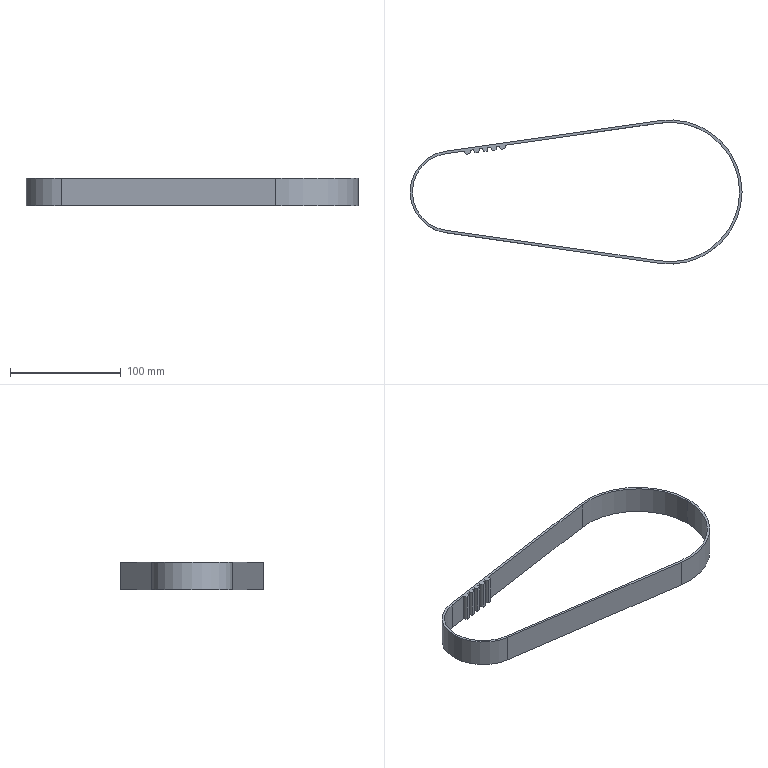Part | SolidWorks | features BaseBody 1 | 1 solid | 37 faces | box 300.461 x 130.452 x 25 mm | volume 41947 mm3 | cylinder 21 | plane 16 | commonest cylinder face diameters 10.4 x15 125.952 x2 130.452 x2 69.929 x1 74.429 x1
STEP:
#1=CARTESIAN_POINT('',(188.793,-64.57,-12.5));
#2=VERTEX_POINT('',#1);
#3=CARTESIAN_POINT('',(263.246,0.,-12.5));
#4=VERTEX_POINT('',#3);
#5=CARTESIAN_POINT('',(198.02,0.,-12.5));
#6=DIRECTION('',(0.,0.,1.));
#7=DIRECTION('',(1.,0.,0.));
#8=AXIS2_PLACEMENT_3D('',#5,#6,#7);
#9=CIRCLE('',#8,65.226);
#10=EDGE_CURVE('',#2,#4,#9,.T.);
#11=ORIENTED_EDGE('',*,*,#10,.T.);
#12=CARTESIAN_POINT('',(263.246,0.,12.5));
#13=VERTEX_POINT('',#12);
#14=CARTESIAN_POINT('',(263.246,0.,12.5));
#15=DIRECTION('',(0.,0.,1.));
#16=VECTOR('',#15,1000.);
#17=LINE('',#14,#16);
#18=EDGE_CURVE('',#4,#13,#17,.T.);
#19=ORIENTED_EDGE('',*,*,#18,.T.);
#20=CARTESIAN_POINT('',(188.793,-64.57,12.5));
#21=VERTEX_POINT('',#20);
#22=CARTESIAN_POINT('',(198.02,0.,12.5));
#23=DIRECTION('',(0.,0.,-1.));
#24=DIRECTION('',(1.,0.,0.));
#25=AXIS2_PLACEMENT_3D('',#22,#23,#24);
#26=CIRCLE('',#25,65.226);
#27=EDGE_CURVE('',#13,#21,#26,.T.);
#28=ORIENTED_EDGE('',*,*,#27,.T.);
#29=CARTESIAN_POINT('',(188.793,-64.57,12.5));
#30=DIRECTION('',(0.,0.,-1.));
#31=VECTOR('',#30,1000.);
#32=LINE('',#29,#31);
#33=EDGE_CURVE('',#21,#2,#32,.T.);
#34=ORIENTED_EDGE('',*,*,#33,.T.);
#35=EDGE_LOOP('',(#11,#19,#28,#34));
#36=FACE_OUTER_BOUND('',#35,.T.);
#37=CARTESIAN_POINT('',(198.02,0.,12.5));
#38=DIRECTION('',(0.,0.,1.));
#39=DIRECTION('',(1.,0.,0.));
#40=AXIS2_PLACEMENT_3D('',#37,#38,#39);
#41=CYLINDRICAL_SURFACE('',#40,65.226);
#42=ADVANCED_FACE('',(#36),#41,.T.);
#43=CARTESIAN_POINT('',(189.112,62.343,-12.5));
#44=VERTEX_POINT('',#43);
#45=CARTESIAN_POINT('',(260.996,0.,-12.5));
#46=VERTEX_POINT('',#45);
#47=CARTESIAN_POINT('',(198.02,0.,-12.5));
#48=DIRECTION('',(0.,0.,-1.));
#49=DIRECTION('',(1.,0.,0.));
#50=AXIS2_PLACEMENT_3D('',#47,#48,#49);
#51=CIRCLE('',#50,62.976);
#52=EDGE_CURVE('',#44,#46,#51,.T.);
#53=ORIENTED_EDGE('',*,*,#52,.T.);
#54=CARTESIAN_POINT('',(260.996,0.,12.5));
#55=VERTEX_POINT('',#54);
#56=CARTESIAN_POINT('',(260.996,0.,12.5));
#57=DIRECTION('',(0.,0.,1.));
#58=VECTOR('',#57,1000.);
#59=LINE('',#56,#58);
#60=EDGE_CURVE('',#46,#55,#59,.T.);
#61=ORIENTED_EDGE('',*,*,#60,.T.);
#62=CARTESIAN_POINT('',(189.112,62.343,12.5));
#63=VERTEX_POINT('',#62);
#64=CARTESIAN_POINT('',(198.02,0.,12.5));
#65=DIRECTION('',(0.,0.,-1.));
#66=DIRECTION('',(1.,0.,0.));
#67=AXIS2_PLACEMENT_3D('',#64,#65,#66);
#68=CIRCLE('',#67,62.976);
#69=EDGE_CURVE('',#63,#55,#68,.T.);
#70=ORIENTED_EDGE('',*,*,#69,.F.);
#71=CARTESIAN_POINT('',(189.112,62.343,12.5));
#72=DIRECTION('',(0.,0.,1.));
#73=VECTOR('',#72,1000.);
#74=LINE('',#71,#73);
#75=EDGE_CURVE('',#44,#63,#74,.T.);
#76=ORIENTED_EDGE('',*,*,#75,.F.);
#77=EDGE_LOOP('',(#53,#61,#70,#76));
#78=FACE_OUTER_BOUND('',#77,.T.);
#79=CARTESIAN_POINT('',(198.02,0.,12.5));
#80=DIRECTION('',(0.,0.,1.));
#81=DIRECTION('',(1.,0.,0.));
#82=AXIS2_PLACEMENT_3D('',#79,#80,#81);
#83=CYLINDRICAL_SURFACE('',#82,62.976);
#84=ADVANCED_FACE('',(#78),#83,.F.);
#85=CARTESIAN_POINT('',(48.558,39.178,-12.5));
#86=VERTEX_POINT('',#85);
#87=CARTESIAN_POINT('',(49.157,41.601,-12.5));
#88=VERTEX_POINT('',#87);
#89=CARTESIAN_POINT('',(43.957,41.601,-12.5));
#90=DIRECTION('',(0.,0.,1.));
#91=DIRECTION('',(1.,0.,0.));
#92=AXIS2_PLACEMENT_3D('',#89,#90,#91);
#93=CIRCLE('',#92,5.2);
#94=EDGE_CURVE('',#86,#88,#93,.T.);
#95=ORIENTED_EDGE('',*,*,#94,.T.);
#96=CARTESIAN_POINT('',(49.157,41.601,12.5));
#97=VERTEX_POINT('',#96);
#98=CARTESIAN_POINT('',(49.157,41.601,12.5));
#99=DIRECTION('',(0.,0.,1.));
#100=VECTOR('',#99,1000.);
#101=LINE('',#98,#100);
#102=EDGE_CURVE('',#88,#97,#101,.T.);
#103=ORIENTED_EDGE('',*,*,#102,.T.);
#104=CARTESIAN_POINT('',(48.558,39.178,12.5));
#105=VERTEX_POINT('',#104);
#106=CARTESIAN_POINT('',(43.957,41.601,12.5));
#107=DIRECTION('',(0.,0.,1.));
#108=DIRECTION('',(1.,0.,0.));
#109=AXIS2_PLACEMENT_3D('',#106,#107,#108);
#110=CIRCLE('',#109,5.2);
#111=EDGE_CURVE('',#105,#97,#110,.T.);
#112=ORIENTED_EDGE('',*,*,#111,.F.);
#113=CARTESIAN_POINT('',(48.558,39.178,12.5));
#114=DIRECTION('',(0.,0.,-1.));
#115=VECTOR('',#114,1000.);
#116=LINE('',#113,#115);
#117=EDGE_CURVE('',#105,#86,#116,.T.);
#118=ORIENTED_EDGE('',*,*,#117,.T.);
#119=EDGE_LOOP('',(#95,#103,#112,#118));
#120=FACE_OUTER_BOUND('',#119,.T.);
#121=CARTESIAN_POINT('',(43.957,41.601,12.5));
#122=DIRECTION('',(0.,0.,1.));
#123=DIRECTION('',(1.,0.,0.));
#124=AXIS2_PLACEMENT_3D('',#121,#122,#123);
#125=CYLINDRICAL_SURFACE('',#124,5.2);
#126=ADVANCED_FACE('',(#120),#125,.T.);
#127=CARTESIAN_POINT('',(40.638,38.046,-12.5));
#128=VERTEX_POINT('',#127);
#129=CARTESIAN_POINT('',(41.238,40.469,-12.5));
#130=VERTEX_POINT('',#129);
#131=CARTESIAN_POINT('',(36.038,40.469,-12.5));
#132=DIRECTION('',(0.,0.,1.));
#133=DIRECTION('',(1.,0.,0.));
#134=AXIS2_PLACEMENT_3D('',#131,#132,#133);
#135=CIRCLE('',#134,5.2);
#136=EDGE_CURVE('',#128,#130,#135,.T.);
#137=ORIENTED_EDGE('',*,*,#136,.T.);
#138=CARTESIAN_POINT('',(41.238,40.469,12.5));
#139=VERTEX_POINT('',#138);
#140=CARTESIAN_POINT('',(41.238,40.469,12.5));
#141=DIRECTION('',(0.,0.,1.));
#142=VECTOR('',#141,1000.);
#143=LINE('',#140,#142);
#144=EDGE_CURVE('',#130,#139,#143,.T.);
#145=ORIENTED_EDGE('',*,*,#144,.T.);
#146=CARTESIAN_POINT('',(40.638,38.046,12.5));
#147=VERTEX_POINT('',#146);
#148=CARTESIAN_POINT('',(36.038,40.469,12.5));
#149=DIRECTION('',(0.,0.,1.));
#150=DIRECTION('',(1.,0.,0.));
#151=AXIS2_PLACEMENT_3D('',#148,#149,#150);
#152=CIRCLE('',#151,5.2);
#153=EDGE_CURVE('',#147,#139,#152,.T.);
#154=ORIENTED_EDGE('',*,*,#153,.F.);
#155=CARTESIAN_POINT('',(40.638,38.046,12.5));
#156=DIRECTION('',(0.,0.,-1.));
#157=VECTOR('',#156,1000.);
#158=LINE('',#155,#157);
#159=EDGE_CURVE('',#147,#128,#158,.T.);
#160=ORIENTED_EDGE('',*,*,#159,.T.);
#161=EDGE_LOOP('',(#137,#145,#154,#160));
#162=FACE_OUTER_BOUND('',#161,.T.);
#163=CARTESIAN_POINT('',(36.038,40.469,12.5));
#164=DIRECTION('',(0.,0.,1.));
#165=DIRECTION('',(1.,0.,0.));
#166=AXIS2_PLACEMENT_3D('',#163,#164,#165);
#167=CYLINDRICAL_SURFACE('',#166,5.2);
#168=ADVANCED_FACE('',(#162),#167,.T.);
#169=CARTESIAN_POINT('',(32.719,36.914,-12.5));
#170=VERTEX_POINT('',#169);
#171=CARTESIAN_POINT('',(33.318,39.338,-12.5));
#172=VERTEX_POINT('',#171);
#173=CARTESIAN_POINT('',(28.118,39.338,-12.5));
#174=DIRECTION('',(0.,0.,1.));
#175=DIRECTION('',(1.,0.,0.));
#176=AXIS2_PLACEMENT_3D('',#173,#174,#175);
#177=CIRCLE('',#176,5.2);
#178=EDGE_CURVE('',#170,#172,#177,.T.);
#179=ORIENTED_EDGE('',*,*,#178,.T.);
#180=CARTESIAN_POINT('',(33.318,39.338,12.5));
#181=VERTEX_POINT('',#180);
#182=CARTESIAN_POINT('',(33.318,39.338,12.5));
#183=DIRECTION('',(0.,0.,1.));
#184=VECTOR('',#183,1000.);
#185=LINE('',#182,#184);
#186=EDGE_CURVE('',#172,#181,#185,.T.);
#187=ORIENTED_EDGE('',*,*,#186,.T.);
#188=CARTESIAN_POINT('',(32.719,36.914,12.5));
#189=VERTEX_POINT('',#188);
#190=CARTESIAN_POINT('',(28.118,39.338,12.5));
#191=DIRECTION('',(0.,0.,1.));
#192=DIRECTION('',(1.,0.,0.));
#193=AXIS2_PLACEMENT_3D('',#190,#191,#192);
#194=CIRCLE('',#193,5.2);
#195=EDGE_CURVE('',#189,#181,#194,.T.);
#196=ORIENTED_EDGE('',*,*,#195,.F.);
#197=CARTESIAN_POINT('',(32.719,36.914,12.5));
#198=DIRECTION('',(0.,0.,-1.));
#199=VECTOR('',#198,1000.);
#200=LINE('',#197,#199);
#201=EDGE_CURVE('',#189,#170,#200,.T.);
#202=ORIENTED_EDGE('',*,*,#201,.T.);
#203=EDGE_LOOP('',(#179,#187,#196,#202));
#204=FACE_OUTER_BOUND('',#203,.T.);
#205=CARTESIAN_POINT('',(28.118,39.338,12.5));
#206=DIRECTION('',(0.,0.,1.));
#207=DIRECTION('',(1.,0.,0.));
#208=AXIS2_PLACEMENT_3D('',#205,#206,#207);
#209=CYLINDRICAL_SURFACE('',#208,5.2);
#210=ADVANCED_FACE('',(#204),#209,.T.);
#211=CARTESIAN_POINT('',(24.799,35.783,-12.5));
#212=VERTEX_POINT('',#211);
#213=CARTESIAN_POINT('',(25.399,38.206,-12.5));
#214=VERTEX_POINT('',#213);
#215=CARTESIAN_POINT('',(20.199,38.206,-12.5));
#216=DIRECTION('',(0.,0.,1.));
#217=DIRECTION('',(1.,0.,0.));
#218=AXIS2_PLACEMENT_3D('',#215,#216,#217);
#219=CIRCLE('',#218,5.2);
#220=EDGE_CURVE('',#212,#214,#219,.T.);
#221=ORIENTED_EDGE('',*,*,#220,.T.);
#222=CARTESIAN_POINT('',(25.399,38.206,12.5));
#223=VERTEX_POINT('',#222);
#224=CARTESIAN_POINT('',(25.399,38.206,12.5));
#225=DIRECTION('',(0.,0.,1.));
#226=VECTOR('',#225,1000.);
#227=LINE('',#224,#226);
#228=EDGE_CURVE('',#214,#223,#227,.T.);
#229=ORIENTED_EDGE('',*,*,#228,.T.);
#230=CARTESIAN_POINT('',(24.799,35.783,12.5));
#231=VERTEX_POINT('',#230);
#232=CARTESIAN_POINT('',(20.199,38.206,12.5));
#233=DIRECTION('',(0.,0.,1.));
#234=DIRECTION('',(1.,0.,0.));
#235=AXIS2_PLACEMENT_3D('',#232,#233,#234);
#236=CIRCLE('',#235,5.2);
#237=EDGE_CURVE('',#231,#223,#236,.T.);
#238=ORIENTED_EDGE('',*,*,#237,.F.);
#239=CARTESIAN_POINT('',(24.799,35.783,12.5));
#240=DIRECTION('',(0.,0.,-1.));
#241=VECTOR('',#240,1000.);
#242=LINE('',#239,#241);
#243=EDGE_CURVE('',#231,#212,#242,.T.);
#244=ORIENTED_EDGE('',*,*,#243,.T.);
#245=EDGE_LOOP('',(#221,#229,#238,#244));
#246=FACE_OUTER_BOUND('',#245,.T.);
#247=CARTESIAN_POINT('',(20.199,38.206,12.5));
#248=DIRECTION('',(0.,0.,1.));
#249=DIRECTION('',(1.,0.,0.));
#250=AXIS2_PLACEMENT_3D('',#247,#248,#249);
#251=CYLINDRICAL_SURFACE('',#250,5.2);
#252=ADVANCED_FACE('',(#246),#251,.T.);
#253=CARTESIAN_POINT('',(16.88,34.651,-12.5));
#254=VERTEX_POINT('',#253);
#255=CARTESIAN_POINT('',(17.479,37.074,-12.5));
#256=VERTEX_POINT('',#255);
#257=CARTESIAN_POINT('',(12.279,37.074,-12.5));
#258=DIRECTION('',(0.,0.,1.));
#259=DIRECTION('',(1.,0.,0.));
#260=AXIS2_PLACEMENT_3D('',#257,#258,#259);
#261=CIRCLE('',#260,5.2);
#262=EDGE_CURVE('',#254,#256,#261,.T.);
#263=ORIENTED_EDGE('',*,*,#262,.T.);
#264=CARTESIAN_POINT('',(17.479,37.074,12.5));
#265=VERTEX_POINT('',#264);
#266=CARTESIAN_POINT('',(17.479,37.074,12.5));
#267=DIRECTION('',(0.,0.,1.));
#268=VECTOR('',#267,1000.);
#269=LINE('',#266,#268);
#270=EDGE_CURVE('',#256,#265,#269,.T.);
#271=ORIENTED_EDGE('',*,*,#270,.T.);
#272=CARTESIAN_POINT('',(16.88,34.651,12.5));
#273=VERTEX_POINT('',#272);
#274=CARTESIAN_POINT('',(12.279,37.074,12.5));
#275=DIRECTION('',(0.,0.,1.));
#276=DIRECTION('',(1.,0.,0.));
#277=AXIS2_PLACEMENT_3D('',#274,#275,#276);
#278=CIRCLE('',#277,5.2);
#279=EDGE_CURVE('',#273,#265,#278,.T.);
#280=ORIENTED_EDGE('',*,*,#279,.F.);
#281=CARTESIAN_POINT('',(16.88,34.651,12.5));
#282=DIRECTION('',(0.,0.,-1.));
#283=VECTOR('',#282,1000.);
#284=LINE('',#281,#283);
#285=EDGE_CURVE('',#273,#254,#284,.T.);
#286=ORIENTED_EDGE('',*,*,#285,.T.);
#287=EDGE_LOOP('',(#263,#271,#280,#286));
#288=FACE_OUTER_BOUND('',#287,.T.);
#289=CARTESIAN_POINT('',(12.279,37.074,12.5));
#290=DIRECTION('',(0.,0.,1.));
#291=DIRECTION('',(1.,0.,0.));
#292=AXIS2_PLACEMENT_3D('',#289,#290,#291);
#293=CYLINDRICAL_SURFACE('',#292,5.2);
#294=ADVANCED_FACE('',(#288),#293,.T.);
#295=ORIENTED_EDGE('',*,*,#18,.F.);
#296=CARTESIAN_POINT('',(188.793,64.57,-12.5));
#297=VERTEX_POINT('',#296);
#298=CARTESIAN_POINT('',(198.02,0.,-12.5));
#299=DIRECTION('',(0.,0.,1.));
#300=DIRECTION('',(1.,0.,0.));
#301=AXIS2_PLACEMENT_3D('',#298,#299,#300);
#302=CIRCLE('',#301,65.226);
#303=EDGE_CURVE('',#4,#297,#302,.T.);
#304=ORIENTED_EDGE('',*,*,#303,.T.);
#305=CARTESIAN_POINT('',(188.793,64.57,12.5));
#306=VERTEX_POINT('',#305);
#307=CARTESIAN_POINT('',(188.793,64.57,12.5));
#308=DIRECTION('',(0.,0.,1.));
#309=VECTOR('',#308,1000.);
#310=LINE('',#307,#309);
#311=EDGE_CURVE('',#297,#306,#310,.T.);
#312=ORIENTED_EDGE('',*,*,#311,.T.);
#313=CARTESIAN_POINT('',(198.02,0.,12.5));
#314=DIRECTION('',(0.,0.,-1.));
#315=DIRECTION('',(1.,0.,0.));
#316=AXIS2_PLACEMENT_3D('',#313,#314,#315);
#317=CIRCLE('',#316,65.226);
#318=EDGE_CURVE('',#306,#13,#317,.T.);
#319=ORIENTED_EDGE('',*,*,#318,.T.);
#320=EDGE_LOOP('',(#295,#304,#312,#319));
#321=FACE_OUTER_BOUND('',#320,.T.);
#322=CARTESIAN_POINT('',(198.02,0.,12.5));
#323=DIRECTION('',(0.,0.,1.));
#324=DIRECTION('',(1.,0.,0.));
#325=AXIS2_PLACEMENT_3D('',#322,#323,#324);
#326=CYLINDRICAL_SURFACE('',#325,65.226);
#327=ADVANCED_FACE('',(#321),#326,.T.);
#328=ORIENTED_EDGE('',*,*,#33,.F.);
#329=CARTESIAN_POINT('',(-5.264,-36.84,12.5));
#330=VERTEX_POINT('',#329);
#331=CARTESIAN_POINT('',(-5.264,-36.84,12.5));
#332=DIRECTION('',(0.9899,-0.1415,0.));
#333=VECTOR('',#332,1000.);
#334=LINE('',#331,#333);
#335=EDGE_CURVE('',#330,#21,#334,.T.);
#336=ORIENTED_EDGE('',*,*,#335,.F.);
#337=CARTESIAN_POINT('',(-5.264,-36.84,-12.5));
#338=VERTEX_POINT('',#337);
#339=CARTESIAN_POINT('',(-5.264,-36.84,12.5));
#340=DIRECTION('',(0.,0.,1.));
#341=VECTOR('',#340,1000.);
#342=LINE('',#339,#341);
#343=EDGE_CURVE('',#338,#330,#342,.T.);
#344=ORIENTED_EDGE('',*,*,#343,.F.);
#345=CARTESIAN_POINT('',(-5.264,-36.84,-12.5));
#346=DIRECTION('',(-0.9899,0.1415,0.));
#347=VECTOR('',#346,1000.);
#348=LINE('',#345,#347);
#349=EDGE_CURVE('',#2,#338,#348,.T.);
#350=ORIENTED_EDGE('',*,*,#349,.F.);
#351=EDGE_LOOP('',(#328,#336,#344,#350));
#352=FACE_OUTER_BOUND('',#351,.T.);
#353=CARTESIAN_POINT('',(-5.264,-36.84,12.5));
#354=DIRECTION('',(0.1415,0.9899,0.));
#355=DIRECTION('',(-0.9899,0.1415,0.));
#356=AXIS2_PLACEMENT_3D('',#353,#354,#355);
#357=PLANE('',#356);
#358=ADVANCED_FACE('',(#352),#357,.F.);
#359=CARTESIAN_POINT('',(189.112,-62.343,12.5));
#360=VERTEX_POINT('',#359);
#361=CARTESIAN_POINT('',(-4.946,-34.613,12.5));
#362=VERTEX_POINT('',#361);
#363=CARTESIAN_POINT('',(189.112,-62.343,12.5));
#364=DIRECTION('',(-0.9899,0.1415,0.));
#365=VECTOR('',#364,1000.);
#366=LINE('',#363,#365);
#367=EDGE_CURVE('',#360,#362,#366,.T.);
#368=ORIENTED_EDGE('',*,*,#367,.T.);
#369=CARTESIAN_POINT('',(-4.946,34.613,12.5));
#370=VERTEX_POINT('',#369);
#371=CARTESIAN_POINT('',(0.,0.,12.5));
#372=DIRECTION('',(0.,0.,-1.));
#373=DIRECTION('',(1.,0.,0.));
#374=AXIS2_PLACEMENT_3D('',#371,#372,#373);
#375=CIRCLE('',#374,34.965);
#376=EDGE_CURVE('',#362,#370,#375,.T.);
#377=ORIENTED_EDGE('',*,*,#376,.T.);
#378=CARTESIAN_POINT('',(12.279,37.074,12.5));
#379=VERTEX_POINT('',#378);
#380=CARTESIAN_POINT('',(-4.946,34.613,12.5));
#381=DIRECTION('',(0.9899,0.1415,0.));
#382=VECTOR('',#381,1000.);
#383=LINE('',#380,#382);
#384=EDGE_CURVE('',#370,#379,#383,.T.);
#385=ORIENTED_EDGE('',*,*,#384,.T.);
#386=CARTESIAN_POINT('',(13.689,34.195,12.5));
#387=VERTEX_POINT('',#386);
#388=CARTESIAN_POINT('',(17.427,37.81,12.5));
#389=DIRECTION('',(0.,0.,1.));
#390=DIRECTION('',(1.,0.,0.));
#391=AXIS2_PLACEMENT_3D('',#388,#389,#390);
#392=CIRCLE('',#391,5.2);
#393=EDGE_CURVE('',#379,#387,#392,.T.);
#394=ORIENTED_EDGE('',*,*,#393,.T.);
#395=CARTESIAN_POINT('',(13.689,34.195,12.5));
#396=DIRECTION('',(0.9899,0.1415,0.));
#397=VECTOR('',#396,1000.);
#398=LINE('',#395,#397);
#399=EDGE_CURVE('',#387,#273,#398,.T.);
#400=ORIENTED_EDGE('',*,*,#399,.T.);
#401=ORIENTED_EDGE('',*,*,#279,.T.);
#402=CARTESIAN_POINT('',(17.427,37.81,12.5));
#403=VERTEX_POINT('',#402);
#404=CARTESIAN_POINT('',(12.279,37.074,12.5));
#405=DIRECTION('',(0.,0.,1.));
#406=DIRECTION('',(1.,0.,0.));
#407=AXIS2_PLACEMENT_3D('',#404,#405,#406);
#408=CIRCLE('',#407,5.2);
#409=EDGE_CURVE('',#265,#403,#408,.T.);
#410=ORIENTED_EDGE('',*,*,#409,.T.);
#411=CARTESIAN_POINT('',(20.199,38.206,12.5));
#412=VERTEX_POINT('',#411);
#413=CARTESIAN_POINT('',(17.427,37.81,12.5));
#414=DIRECTION('',(0.9899,0.1415,0.));
#415=VECTOR('',#414,1000.);
#416=LINE('',#413,#415);
#417=EDGE_CURVE('',#403,#412,#416,.T.);
#418=ORIENTED_EDGE('',*,*,#417,.T.);
#419=CARTESIAN_POINT('',(21.609,35.327,12.5));
#420=VERTEX_POINT('',#419);
#421=CARTESIAN_POINT('',(25.346,38.942,12.5));
#422=DIRECTION('',(0.,0.,1.));
#423=DIRECTION('',(1.,0.,0.));
#424=AXIS2_PLACEMENT_3D('',#421,#422,#423);
#425=CIRCLE('',#424,5.2);
#426=EDGE_CURVE('',#412,#420,#425,.T.);
#427=ORIENTED_EDGE('',*,*,#426,.T.);
#428=CARTESIAN_POINT('',(21.609,35.327,12.5));
#429=DIRECTION('',(0.9899,0.1415,0.));
#430=VECTOR('',#429,1000.);
#431=LINE('',#428,#430);
#432=EDGE_CURVE('',#420,#231,#431,.T.);
#433=ORIENTED_EDGE('',*,*,#432,.T.);
#434=ORIENTED_EDGE('',*,*,#237,.T.);
#435=CARTESIAN_POINT('',(25.346,38.942,12.5));
#436=VERTEX_POINT('',#435);
#437=CARTESIAN_POINT('',(20.199,38.206,12.5));
#438=DIRECTION('',(0.,0.,1.));
#439=DIRECTION('',(1.,0.,0.));
#440=AXIS2_PLACEMENT_3D('',#437,#438,#439);
#441=CIRCLE('',#440,5.2);
#442=EDGE_CURVE('',#223,#436,#441,.T.);
#443=ORIENTED_EDGE('',*,*,#442,.T.);
#444=CARTESIAN_POINT('',(28.118,39.338,12.5));
#445=VERTEX_POINT('',#444);
#446=CARTESIAN_POINT('',(25.346,38.942,12.5));
#447=DIRECTION('',(0.9899,0.1415,0.));
#448=VECTOR('',#447,1000.);
#449=LINE('',#446,#448);
#450=EDGE_CURVE('',#436,#445,#449,.T.);
#451=ORIENTED_EDGE('',*,*,#450,.T.);
#452=CARTESIAN_POINT('',(29.528,36.458,12.5));
#453=VERTEX_POINT('',#452);
#454=CARTESIAN_POINT('',(33.266,40.073,12.5));
#455=DIRECTION('',(0.,0.,1.));
#456=DIRECTION('',(1.,0.,0.));
#457=AXIS2_PLACEMENT_3D('',#454,#455,#456);
#458=CIRCLE('',#457,5.2);
#459=EDGE_CURVE('',#445,#453,#458,.T.);
#460=ORIENTED_EDGE('',*,*,#459,.T.);
#461=CARTESIAN_POINT('',(29.528,36.458,12.5));
#462=DIRECTION('',(0.9899,0.1415,0.));
#463=VECTOR('',#462,1000.);
#464=LINE('',#461,#463);
#465=EDGE_CURVE('',#453,#189,#464,.T.);
#466=ORIENTED_EDGE('',*,*,#465,.T.);
#467=ORIENTED_EDGE('',*,*,#195,.T.);
#468=CARTESIAN_POINT('',(33.266,40.073,12.5));
#469=VERTEX_POINT('',#468);
#470=CARTESIAN_POINT('',(28.118,39.338,12.5));
#471=DIRECTION('',(0.,0.,1.));
#472=DIRECTION('',(1.,0.,0.));
#473=AXIS2_PLACEMENT_3D('',#470,#471,#472);
#474=CIRCLE('',#473,5.2);
#475=EDGE_CURVE('',#181,#469,#474,.T.);
#476=ORIENTED_EDGE('',*,*,#475,.T.);
#477=CARTESIAN_POINT('',(36.038,40.469,12.5));
#478=VERTEX_POINT('',#477);
#479=CARTESIAN_POINT('',(33.266,40.073,12.5));
#480=DIRECTION('',(0.9899,0.1415,0.));
#481=VECTOR('',#480,1000.);
#482=LINE('',#479,#481);
#483=EDGE_CURVE('',#469,#478,#482,.T.);
#484=ORIENTED_EDGE('',*,*,#483,.T.);
#485=CARTESIAN_POINT('',(37.448,37.59,12.5));
#486=VERTEX_POINT('',#485);
#487=CARTESIAN_POINT('',(41.185,41.205,12.5));
#488=DIRECTION('',(0.,0.,1.));
#489=DIRECTION('',(1.,0.,0.));
#490=AXIS2_PLACEMENT_3D('',#487,#488,#489);
#491=CIRCLE('',#490,5.2);
#492=EDGE_CURVE('',#478,#486,#491,.T.);
#493=ORIENTED_EDGE('',*,*,#492,.T.);
#494=CARTESIAN_POINT('',(37.448,37.59,12.5));
#495=DIRECTION('',(0.9899,0.1415,0.));
#496=VECTOR('',#495,1000.);
#497=LINE('',#494,#496);
#498=EDGE_CURVE('',#486,#147,#497,.T.);
#499=ORIENTED_EDGE('',*,*,#498,.T.);
#500=ORIENTED_EDGE('',*,*,#153,.T.);
#501=CARTESIAN_POINT('',(41.185,41.205,12.5));
#502=VERTEX_POINT('',#501);
#503=CARTESIAN_POINT('',(36.038,40.469,12.5));
#504=DIRECTION('',(0.,0.,1.));
#505=DIRECTION('',(1.,0.,0.));
#506=AXIS2_PLACEMENT_3D('',#503,#504,#505);
#507=CIRCLE('',#506,5.2);
#508=EDGE_CURVE('',#139,#502,#507,.T.);
#509=ORIENTED_EDGE('',*,*,#508,.T.);
#510=CARTESIAN_POINT('',(43.957,41.601,12.5));
#511=VERTEX_POINT('',#510);
#512=CARTESIAN_POINT('',(41.185,41.205,12.5));
#513=DIRECTION('',(0.9899,0.1415,0.));
#514=VECTOR('',#513,1000.);
#515=LINE('',#512,#514);
#516=EDGE_CURVE('',#502,#511,#515,.T.);
#517=ORIENTED_EDGE('',*,*,#516,.T.);
#518=CARTESIAN_POINT('',(45.367,38.722,12.5));
#519=VERTEX_POINT('',#518);
#520=CARTESIAN_POINT('',(49.105,42.337,12.5));
#521=DIRECTION('',(0.,0.,1.));
#522=DIRECTION('',(1.,0.,0.));
#523=AXIS2_PLACEMENT_3D('',#520,#521,#522);
#524=CIRCLE('',#523,5.2);
#525=EDGE_CURVE('',#511,#519,#524,.T.);
#526=ORIENTED_EDGE('',*,*,#525,.T.);
#527=CARTESIAN_POINT('',(45.367,38.722,12.5));
#528=DIRECTION('',(0.9899,0.1415,0.));
#529=VECTOR('',#528,1000.);
#530=LINE('',#527,#529);
#531=EDGE_CURVE('',#519,#105,#530,.T.);
#532=ORIENTED_EDGE('',*,*,#531,.T.);
#533=ORIENTED_EDGE('',*,*,#111,.T.);
#534=CARTESIAN_POINT('',(49.105,42.337,12.5));
#535=VERTEX_POINT('',#534);
#536=CARTESIAN_POINT('',(43.957,41.601,12.5));
#537=DIRECTION('',(0.,0.,1.));
#538=DIRECTION('',(1.,0.,0.));
#539=AXIS2_PLACEMENT_3D('',#536,#537,#538);
#540=CIRCLE('',#539,5.2);
#541=EDGE_CURVE('',#97,#535,#540,.T.);
#542=ORIENTED_EDGE('',*,*,#541,.T.);
#543=CARTESIAN_POINT('',(49.105,42.337,12.5));
#544=DIRECTION('',(0.9899,0.1415,0.));
#545=VECTOR('',#544,1000.);
#546=LINE('',#543,#545);
#547=EDGE_CURVE('',#535,#63,#546,.T.);
#548=ORIENTED_EDGE('',*,*,#547,.T.);
#549=ORIENTED_EDGE('',*,*,#69,.T.);
#550=CARTESIAN_POINT('',(198.02,0.,12.5));
#551=DIRECTION('',(0.,0.,-1.));
#552=DIRECTION('',(1.,0.,0.));
#553=AXIS2_PLACEMENT_3D('',#550,#551,#552);
#554=CIRCLE('',#553,62.976);
#555=EDGE_CURVE('',#55,#360,#554,.T.);
#556=ORIENTED_EDGE('',*,*,#555,.T.);
#557=EDGE_LOOP('',(#368,#377,#385,#394,#400,#401,#410,#418,#427,#433,#434,#443,#451,#460,#466,#467,#476,#484,#493,#499,#500,#509,#517,#526,#532,#533,#542,#548,#549,#556));
#558=FACE_BOUND('',#557,.T.);
#559=ORIENTED_EDGE('',*,*,#335,.T.);
#560=ORIENTED_EDGE('',*,*,#27,.F.);
#561=ORIENTED_EDGE('',*,*,#318,.F.);
#562=CARTESIAN_POINT('',(-5.264,36.84,12.5));
#563=VERTEX_POINT('',#562);
#564=CARTESIAN_POINT('',(188.793,64.57,12.5));
#565=DIRECTION('',(-0.9899,-0.1415,0.));
#566=VECTOR('',#565,1000.);
#567=LINE('',#564,#566);
#568=EDGE_CURVE('',#306,#563,#567,.T.);
#569=ORIENTED_EDGE('',*,*,#568,.T.);
#570=CARTESIAN_POINT('',(0.,0.,12.5));
#571=DIRECTION('',(0.,0.,1.));
#572=DIRECTION('',(1.,0.,0.));
#573=AXIS2_PLACEMENT_3D('',#570,#571,#572);
#574=CIRCLE('',#573,37.215);
#575=EDGE_CURVE('',#563,#330,#574,.T.);
#576=ORIENTED_EDGE('',*,*,#575,.T.);
#577=EDGE_LOOP('',(#559,#560,#561,#569,#576));
#578=FACE_OUTER_BOUND('',#577,.T.);
#579=CARTESIAN_POINT('',(17.427,37.81,12.5));
#580=DIRECTION('',(0.,0.,1.));
#581=DIRECTION('',(1.,0.,0.));
#582=AXIS2_PLACEMENT_3D('',#579,#580,#581);
#583=PLANE('',#582);
#584=ADVANCED_FACE('',(#558,#578),#583,.T.);
#585=CARTESIAN_POINT('',(-5.264,36.84,-12.5));
#586=VERTEX_POINT('',#585);
#587=CARTESIAN_POINT('',(-5.264,36.84,12.5));
#588=DIRECTION('',(0.,0.,-1.));
#589=VECTOR('',#588,1000.);
#590=LINE('',#587,#589);
#591=EDGE_CURVE('',#563,#586,#590,.T.);
#592=ORIENTED_EDGE('',*,*,#591,.F.);
#593=ORIENTED_EDGE('',*,*,#568,.F.);
#594=ORIENTED_EDGE('',*,*,#311,.F.);
#595=CARTESIAN_POINT('',(50.173,44.762,-12.5));
#596=DIRECTION('',(0.9899,0.1415,0.));
#597=VECTOR('',#596,1000.);
#598=LINE('',#595,#597);
#599=EDGE_CURVE('',#586,#297,#598,.T.);
#600=ORIENTED_EDGE('',*,*,#599,.F.);
#601=EDGE_LOOP('',(#592,#593,#594,#600));
#602=FACE_OUTER_BOUND('',#601,.T.);
#603=CARTESIAN_POINT('',(50.173,44.762,12.5));
#604=DIRECTION('',(0.1415,-0.9899,0.));
#605=DIRECTION('',(0.9899,0.1415,0.));
#606=AXIS2_PLACEMENT_3D('',#603,#604,#605);
#607=PLANE('',#606);
#608=ADVANCED_FACE('',(#602),#607,.F.);
#609=CARTESIAN_POINT('',(-4.946,-34.613,-12.5));
#610=VERTEX_POINT('',#609);
#611=CARTESIAN_POINT('',(-4.946,34.613,-12.5));
#612=VERTEX_POINT('',#611);
#613=CARTESIAN_POINT('',(0.,0.,-12.5));
#614=DIRECTION('',(0.,0.,-1.));
#615=DIRECTION('',(1.,0.,0.));
#616=AXIS2_PLACEMENT_3D('',#613,#614,#615);
#617=CIRCLE('',#616,34.965);
#618=EDGE_CURVE('',#610,#612,#617,.T.);
#619=ORIENTED_EDGE('',*,*,#618,.F.);
#620=CARTESIAN_POINT('',(189.112,-62.343,-12.5));
#621=VERTEX_POINT('',#620);
#622=CARTESIAN_POINT('',(189.112,-62.343,-12.5));
#623=DIRECTION('',(-0.9899,0.1415,0.));
#624=VECTOR('',#623,1000.);
#625=LINE('',#622,#624);
#626=EDGE_CURVE('',#621,#610,#625,.T.);
#627=ORIENTED_EDGE('',*,*,#626,.F.);
#628=CARTESIAN_POINT('',(198.02,0.,-12.5));
#629=DIRECTION('',(0.,0.,-1.));
#630=DIRECTION('',(1.,0.,0.));
#631=AXIS2_PLACEMENT_3D('',#628,#629,#630);
#632=CIRCLE('',#631,62.976);
#633=EDGE_CURVE('',#46,#621,#632,.T.);
#634=ORIENTED_EDGE('',*,*,#633,.F.);
#635=ORIENTED_EDGE('',*,*,#52,.F.);
#636=CARTESIAN_POINT('',(49.105,42.337,-12.5));
#637=VERTEX_POINT('',#636);
#638=CARTESIAN_POINT('',(49.105,42.337,-12.5));
#639=DIRECTION('',(0.9899,0.1415,0.));
#640=VECTOR('',#639,1000.);
#641=LINE('',#638,#640);
#642=EDGE_CURVE('',#637,#44,#641,.T.);
#643=ORIENTED_EDGE('',*,*,#642,.F.);
#644=CARTESIAN_POINT('',(43.957,41.601,-12.5));
#645=DIRECTION('',(0.,0.,1.));
#646=DIRECTION('',(1.,0.,0.));
#647=AXIS2_PLACEMENT_3D('',#644,#645,#646);
#648=CIRCLE('',#647,5.2);
#649=EDGE_CURVE('',#88,#637,#648,.T.);
#650=ORIENTED_EDGE('',*,*,#649,.F.);
#651=ORIENTED_EDGE('',*,*,#94,.F.);
#652=CARTESIAN_POINT('',(45.367,38.722,-12.5));
#653=VERTEX_POINT('',#652);
#654=CARTESIAN_POINT('',(45.367,38.722,-12.5));
#655=DIRECTION('',(0.9899,0.1415,0.));
#656=VECTOR('',#655,1000.);
#657=LINE('',#654,#656);
#658=EDGE_CURVE('',#653,#86,#657,.T.);
#659=ORIENTED_EDGE('',*,*,#658,.F.);
#660=CARTESIAN_POINT('',(43.957,41.601,-12.5));
#661=VERTEX_POINT('',#660);
#662=CARTESIAN_POINT('',(49.105,42.337,-12.5));
#663=DIRECTION('',(0.,0.,1.));
#664=DIRECTION('',(1.,0.,0.));
#665=AXIS2_PLACEMENT_3D('',#662,#663,#664);
#666=CIRCLE('',#665,5.2);
#667=EDGE_CURVE('',#661,#653,#666,.T.);
#668=ORIENTED_EDGE('',*,*,#667,.F.);
#669=CARTESIAN_POINT('',(41.185,41.205,-12.5));
#670=VERTEX_POINT('',#669);
#671=CARTESIAN_POINT('',(41.185,41.205,-12.5));
#672=DIRECTION('',(0.9899,0.1415,0.));
#673=VECTOR('',#672,1000.);
#674=LINE('',#671,#673);
#675=EDGE_CURVE('',#670,#661,#674,.T.);
#676=ORIENTED_EDGE('',*,*,#675,.F.);
#677=CARTESIAN_POINT('',(36.038,40.469,-12.5));
#678=DIRECTION('',(0.,0.,1.));
#679=DIRECTION('',(1.,0.,0.));
#680=AXIS2_PLACEMENT_3D('',#677,#678,#679);
#681=CIRCLE('',#680,5.2);
#682=EDGE_CURVE('',#130,#670,#681,.T.);
#683=ORIENTED_EDGE('',*,*,#682,.F.);
#684=ORIENTED_EDGE('',*,*,#136,.F.);
#685=CARTESIAN_POINT('',(37.448,37.59,-12.5));
#686=VERTEX_POINT('',#685);
#687=CARTESIAN_POINT('',(37.448,37.59,-12.5));
#688=DIRECTION('',(0.9899,0.1415,0.));
#689=VECTOR('',#688,1000.);
#690=LINE('',#687,#689);
#691=EDGE_CURVE('',#686,#128,#690,.T.);
#692=ORIENTED_EDGE('',*,*,#691,.F.);
#693=CARTESIAN_POINT('',(36.038,40.469,-12.5));
#694=VERTEX_POINT('',#693);
#695=CARTESIAN_POINT('',(41.185,41.205,-12.5));
#696=DIRECTION('',(0.,0.,1.));
#697=DIRECTION('',(1.,0.,0.));
#698=AXIS2_PLACEMENT_3D('',#695,#696,#697);
#699=CIRCLE('',#698,5.2);
#700=EDGE_CURVE('',#694,#686,#699,.T.);
#701=ORIENTED_EDGE('',*,*,#700,.F.);
#702=CARTESIAN_POINT('',(33.266,40.073,-12.5));
#703=VERTEX_POINT('',#702);
#704=CARTESIAN_POINT('',(33.266,40.073,-12.5));
#705=DIRECTION('',(0.9899,0.1415,0.));
#706=VECTOR('',#705,1000.);
#707=LINE('',#704,#706);
#708=EDGE_CURVE('',#703,#694,#707,.T.);
#709=ORIENTED_EDGE('',*,*,#708,.F.);
#710=CARTESIAN_POINT('',(28.118,39.338,-12.5));
#711=DIRECTION('',(0.,0.,1.));
#712=DIRECTION('',(1.,0.,0.));
#713=AXIS2_PLACEMENT_3D('',#710,#711,#712);
#714=CIRCLE('',#713,5.2);
#715=EDGE_CURVE('',#172,#703,#714,.T.);
#716=ORIENTED_EDGE('',*,*,#715,.F.);
#717=ORIENTED_EDGE('',*,*,#178,.F.);
#718=CARTESIAN_POINT('',(29.528,36.458,-12.5));
#719=VERTEX_POINT('',#718);
#720=CARTESIAN_POINT('',(29.528,36.458,-12.5));
#721=DIRECTION('',(0.9899,0.1415,0.));
#722=VECTOR('',#721,1000.);
#723=LINE('',#720,#722);
#724=EDGE_CURVE('',#719,#170,#723,.T.);
#725=ORIENTED_EDGE('',*,*,#724,.F.);
#726=CARTESIAN_POINT('',(28.118,39.338,-12.5));
#727=VERTEX_POINT('',#726);
#728=CARTESIAN_POINT('',(33.266,40.073,-12.5));
#729=DIRECTION('',(0.,0.,1.));
#730=DIRECTION('',(1.,0.,0.));
#731=AXIS2_PLACEMENT_3D('',#728,#729,#730);
#732=CIRCLE('',#731,5.2);
#733=EDGE_CURVE('',#727,#719,#732,.T.);
#734=ORIENTED_EDGE('',*,*,#733,.F.);
#735=CARTESIAN_POINT('',(25.346,38.942,-12.5));
#736=VERTEX_POINT('',#735);
#737=CARTESIAN_POINT('',(25.346,38.942,-12.5));
#738=DIRECTION('',(0.9899,0.1415,0.));
#739=VECTOR('',#738,1000.);
#740=LINE('',#737,#739);
#741=EDGE_CURVE('',#736,#727,#740,.T.);
#742=ORIENTED_EDGE('',*,*,#741,.F.);
#743=CARTESIAN_POINT('',(20.199,38.206,-12.5));
#744=DIRECTION('',(0.,0.,1.));
#745=DIRECTION('',(1.,0.,0.));
#746=AXIS2_PLACEMENT_3D('',#743,#744,#745);
#747=CIRCLE('',#746,5.2);
#748=EDGE_CURVE('',#214,#736,#747,.T.);
#749=ORIENTED_EDGE('',*,*,#748,.F.);
#750=ORIENTED_EDGE('',*,*,#220,.F.);
#751=CARTESIAN_POINT('',(21.609,35.327,-12.5));
#752=VERTEX_POINT('',#751);
#753=CARTESIAN_POINT('',(21.609,35.327,-12.5));
#754=DIRECTION('',(0.9899,0.1415,0.));
#755=VECTOR('',#754,1000.);
#756=LINE('',#753,#755);
#757=EDGE_CURVE('',#752,#212,#756,.T.);
#758=ORIENTED_EDGE('',*,*,#757,.F.);
#759=CARTESIAN_POINT('',(20.199,38.206,-12.5));
#760=VERTEX_POINT('',#759);
#761=CARTESIAN_POINT('',(25.346,38.942,-12.5));
#762=DIRECTION('',(0.,0.,1.));
#763=DIRECTION('',(1.,0.,0.));
#764=AXIS2_PLACEMENT_3D('',#761,#762,#763);
#765=CIRCLE('',#764,5.2);
#766=EDGE_CURVE('',#760,#752,#765,.T.);
#767=ORIENTED_EDGE('',*,*,#766,.F.);
#768=CARTESIAN_POINT('',(17.427,37.81,-12.5));
#769=VERTEX_POINT('',#768);
#770=CARTESIAN_POINT('',(17.427,37.81,-12.5));
#771=DIRECTION('',(0.9899,0.1415,0.));
#772=VECTOR('',#771,1000.);
#773=LINE('',#770,#772);
#774=EDGE_CURVE('',#769,#760,#773,.T.);
#775=ORIENTED_EDGE('',*,*,#774,.F.);
#776=CARTESIAN_POINT('',(12.279,37.074,-12.5));
#777=DIRECTION('',(0.,0.,1.));
#778=DIRECTION('',(1.,0.,0.));
#779=AXIS2_PLACEMENT_3D('',#776,#777,#778);
#780=CIRCLE('',#779,5.2);
#781=EDGE_CURVE('',#256,#769,#780,.T.);
#782=ORIENTED_EDGE('',*,*,#781,.F.);
#783=ORIENTED_EDGE('',*,*,#262,.F.);
#784=CARTESIAN_POINT('',(13.689,34.195,-12.5));
#785=VERTEX_POINT('',#784);
#786=CARTESIAN_POINT('',(13.689,34.195,-12.5));
#787=DIRECTION('',(0.9899,0.1415,0.));
#788=VECTOR('',#787,1000.);
#789=LINE('',#786,#788);
#790=EDGE_CURVE('',#785,#254,#789,.T.);
#791=ORIENTED_EDGE('',*,*,#790,.F.);
#792=CARTESIAN_POINT('',(12.279,37.074,-12.5));
#793=VERTEX_POINT('',#792);
#794=CARTESIAN_POINT('',(17.427,37.81,-12.5));
#795=DIRECTION('',(0.,0.,1.));
#796=DIRECTION('',(1.,0.,0.));
#797=AXIS2_PLACEMENT_3D('',#794,#795,#796);
#798=CIRCLE('',#797,5.2);
#799=EDGE_CURVE('',#793,#785,#798,.T.);
#800=ORIENTED_EDGE('',*,*,#799,.F.);
#801=CARTESIAN_POINT('',(-4.946,34.613,-12.5));
#802=DIRECTION('',(0.9899,0.1415,0.));
#803=VECTOR('',#802,1000.);
#804=LINE('',#801,#803);
#805=EDGE_CURVE('',#612,#793,#804,.T.);
#806=ORIENTED_EDGE('',*,*,#805,.F.);
#807=EDGE_LOOP('',(#619,#627,#634,#635,#643,#650,#651,#659,#668,#676,#683,#684,#692,#701,#709,#716,#717,#725,#734,#742,#749,#750,#758,#767,#775,#782,#783,#791,#800,#806));
#808=FACE_BOUND('',#807,.T.);
#809=ORIENTED_EDGE('',*,*,#599,.T.);
#810=ORIENTED_EDGE('',*,*,#303,.F.);
#811=ORIENTED_EDGE('',*,*,#10,.F.);
#812=ORIENTED_EDGE('',*,*,#349,.T.);
#813=CARTESIAN_POINT('',(0.,0.,-12.5));
#814=DIRECTION('',(0.,0.,1.));
#815=DIRECTION('',(1.,0.,0.));
#816=AXIS2_PLACEMENT_3D('',#813,#814,#815);
#817=CIRCLE('',#816,37.215);
#818=EDGE_CURVE('',#586,#338,#817,.T.);
#819=ORIENTED_EDGE('',*,*,#818,.F.);
#820=EDGE_LOOP('',(#809,#810,#811,#812,#819));
#821=FACE_OUTER_BOUND('',#820,.T.);
#822=CARTESIAN_POINT('',(17.427,37.81,-12.5));
#823=DIRECTION('',(0.,0.,1.));
#824=DIRECTION('',(1.,0.,0.));
#825=AXIS2_PLACEMENT_3D('',#822,#823,#824);
#826=PLANE('',#825);
#827=ADVANCED_FACE('',(#808,#821),#826,.F.);
#828=ORIENTED_EDGE('',*,*,#343,.T.);
#829=ORIENTED_EDGE('',*,*,#575,.F.);
#830=ORIENTED_EDGE('',*,*,#591,.T.);
#831=ORIENTED_EDGE('',*,*,#818,.T.);
#832=EDGE_LOOP('',(#828,#829,#830,#831));
#833=FACE_OUTER_BOUND('',#832,.T.);
#834=CARTESIAN_POINT('',(0.,0.,12.5));
#835=DIRECTION('',(0.,0.,1.));
#836=DIRECTION('',(1.,0.,0.));
#837=AXIS2_PLACEMENT_3D('',#834,#835,#836);
#838=CYLINDRICAL_SURFACE('',#837,37.215);
#839=ADVANCED_FACE('',(#833),#838,.T.);
#840=CARTESIAN_POINT('',(-4.946,-34.613,12.5));
#841=DIRECTION('',(0.,0.,1.));
#842=VECTOR('',#841,1000.);
#843=LINE('',#840,#842);
#844=EDGE_CURVE('',#610,#362,#843,.T.);
#845=ORIENTED_EDGE('',*,*,#844,.F.);
#846=ORIENTED_EDGE('',*,*,#618,.T.);
#847=CARTESIAN_POINT('',(-4.946,34.613,12.5));
#848=DIRECTION('',(0.,0.,1.));
#849=VECTOR('',#848,1000.);
#850=LINE('',#847,#849);
#851=EDGE_CURVE('',#612,#370,#850,.T.);
#852=ORIENTED_EDGE('',*,*,#851,.T.);
#853=ORIENTED_EDGE('',*,*,#376,.F.);
#854=EDGE_LOOP('',(#845,#846,#852,#853));
#855=FACE_OUTER_BOUND('',#854,.T.);
#856=CARTESIAN_POINT('',(0.,0.,12.5));
#857=DIRECTION('',(0.,0.,1.));
#858=DIRECTION('',(1.,0.,0.));
#859=AXIS2_PLACEMENT_3D('',#856,#857,#858);
#860=CYLINDRICAL_SURFACE('',#859,34.965);
#861=ADVANCED_FACE('',(#855),#860,.F.);
#862=ORIENTED_EDGE('',*,*,#367,.F.);
#863=CARTESIAN_POINT('',(189.112,-62.343,12.5));
#864=DIRECTION('',(0.,0.,-1.));
#865=VECTOR('',#864,1000.);
#866=LINE('',#863,#865);
#867=EDGE_CURVE('',#360,#621,#866,.T.);
#868=ORIENTED_EDGE('',*,*,#867,.T.);
#869=ORIENTED_EDGE('',*,*,#626,.T.);
#870=ORIENTED_EDGE('',*,*,#844,.T.);
#871=EDGE_LOOP('',(#862,#868,#869,#870));
#872=FACE_OUTER_BOUND('',#871,.T.);
#873=CARTESIAN_POINT('',(-4.946,-34.613,12.5));
#874=DIRECTION('',(0.1415,0.9899,0.));
#875=DIRECTION('',(-0.9899,0.1415,0.));
#876=AXIS2_PLACEMENT_3D('',#873,#874,#875);
#877=PLANE('',#876);
#878=ADVANCED_FACE('',(#872),#877,.T.);
#879=ORIENTED_EDGE('',*,*,#60,.F.);
#880=ORIENTED_EDGE('',*,*,#633,.T.);
#881=ORIENTED_EDGE('',*,*,#867,.F.);
#882=ORIENTED_EDGE('',*,*,#555,.F.);
#883=EDGE_LOOP('',(#879,#880,#881,#882));
#884=FACE_OUTER_BOUND('',#883,.T.);
#885=CARTESIAN_POINT('',(198.02,0.,12.5));
#886=DIRECTION('',(0.,0.,1.));
#887=DIRECTION('',(1.,0.,0.));
#888=AXIS2_PLACEMENT_3D('',#885,#886,#887);
#889=CYLINDRICAL_SURFACE('',#888,62.976);
#890=ADVANCED_FACE('',(#884),#889,.F.);
#891=ORIENTED_EDGE('',*,*,#75,.T.);
#892=ORIENTED_EDGE('',*,*,#547,.F.);
#893=CARTESIAN_POINT('',(49.105,42.337,12.5));
#894=DIRECTION('',(0.,0.,1.));
#895=VECTOR('',#894,1000.);
#896=LINE('',#893,#895);
#897=EDGE_CURVE('',#637,#535,#896,.T.);
#898=ORIENTED_EDGE('',*,*,#897,.F.);
#899=ORIENTED_EDGE('',*,*,#642,.T.);
#900=EDGE_LOOP('',(#891,#892,#898,#899));
#901=FACE_OUTER_BOUND('',#900,.T.);
#902=CARTESIAN_POINT('',(49.105,42.337,12.5));
#903=DIRECTION('',(-0.1415,0.9899,0.));
#904=DIRECTION('',(-0.9899,-0.1415,0.));
#905=AXIS2_PLACEMENT_3D('',#902,#903,#904);
#906=PLANE('',#905);
#907=ADVANCED_FACE('',(#901),#906,.F.);
#908=ORIENTED_EDGE('',*,*,#102,.F.);
#909=ORIENTED_EDGE('',*,*,#649,.T.);
#910=ORIENTED_EDGE('',*,*,#897,.T.);
#911=ORIENTED_EDGE('',*,*,#541,.F.);
#912=EDGE_LOOP('',(#908,#909,#910,#911));
#913=FACE_OUTER_BOUND('',#912,.T.);
#914=CARTESIAN_POINT('',(43.957,41.601,12.5));
#915=DIRECTION('',(0.,0.,1.));
#916=DIRECTION('',(1.,0.,0.));
#917=AXIS2_PLACEMENT_3D('',#914,#915,#916);
#918=CYLINDRICAL_SURFACE('',#917,5.2);
#919=ADVANCED_FACE('',(#913),#918,.T.);
#920=ORIENTED_EDGE('',*,*,#117,.F.);
#921=ORIENTED_EDGE('',*,*,#531,.F.);
#922=CARTESIAN_POINT('',(45.367,38.722,12.5));
#923=DIRECTION('',(0.,0.,1.));
#924=VECTOR('',#923,1000.);
#925=LINE('',#922,#924);
#926=EDGE_CURVE('',#653,#519,#925,.T.);
#927=ORIENTED_EDGE('',*,*,#926,.F.);
#928=ORIENTED_EDGE('',*,*,#658,.T.);
#929=EDGE_LOOP('',(#920,#921,#927,#928));
#930=FACE_OUTER_BOUND('',#929,.T.);
#931=CARTESIAN_POINT('',(45.367,38.722,12.5));
#932=DIRECTION('',(-0.1415,0.9899,0.));
#933=DIRECTION('',(-0.9899,-0.1415,0.));
#934=AXIS2_PLACEMENT_3D('',#931,#932,#933);
#935=PLANE('',#934);
#936=ADVANCED_FACE('',(#930),#935,.F.);
#937=ORIENTED_EDGE('',*,*,#525,.F.);
#938=CARTESIAN_POINT('',(43.957,41.601,12.5));
#939=DIRECTION('',(0.,0.,-1.));
#940=VECTOR('',#939,1000.);
#941=LINE('',#938,#940);
#942=EDGE_CURVE('',#511,#661,#941,.T.);
#943=ORIENTED_EDGE('',*,*,#942,.T.);
#944=ORIENTED_EDGE('',*,*,#667,.T.);
#945=ORIENTED_EDGE('',*,*,#926,.T.);
#946=EDGE_LOOP('',(#937,#943,#944,#945));
#947=FACE_OUTER_BOUND('',#946,.T.);
#948=CARTESIAN_POINT('',(49.105,42.337,12.5));
#949=DIRECTION('',(0.,0.,1.));
#950=DIRECTION('',(1.,0.,0.));
#951=AXIS2_PLACEMENT_3D('',#948,#949,#950);
#952=CYLINDRICAL_SURFACE('',#951,5.2);
#953=ADVANCED_FACE('',(#947),#952,.T.);
#954=ORIENTED_EDGE('',*,*,#942,.F.);
#955=ORIENTED_EDGE('',*,*,#516,.F.);
#956=CARTESIAN_POINT('',(41.185,41.205,12.5));
#957=DIRECTION('',(0.,0.,1.));
#958=VECTOR('',#957,1000.);
#959=LINE('',#956,#958);
#960=EDGE_CURVE('',#670,#502,#959,.T.);
#961=ORIENTED_EDGE('',*,*,#960,.F.);
#962=ORIENTED_EDGE('',*,*,#675,.T.);
#963=EDGE_LOOP('',(#954,#955,#961,#962));
#964=FACE_OUTER_BOUND('',#963,.T.);
#965=CARTESIAN_POINT('',(41.185,41.205,12.5));
#966=DIRECTION('',(-0.1415,0.9899,0.));
#967=DIRECTION('',(-0.9899,-0.1415,0.));
#968=AXIS2_PLACEMENT_3D('',#965,#966,#967);
#969=PLANE('',#968);
#970=ADVANCED_FACE('',(#964),#969,.F.);
#971=ORIENTED_EDGE('',*,*,#144,.F.);
#972=ORIENTED_EDGE('',*,*,#682,.T.);
#973=ORIENTED_EDGE('',*,*,#960,.T.);
#974=ORIENTED_EDGE('',*,*,#508,.F.);
#975=EDGE_LOOP('',(#971,#972,#973,#974));
#976=FACE_OUTER_BOUND('',#975,.T.);
#977=CARTESIAN_POINT('',(36.038,40.469,12.5));
#978=DIRECTION('',(0.,0.,1.));
#979=DIRECTION('',(1.,0.,0.));
#980=AXIS2_PLACEMENT_3D('',#977,#978,#979);
#981=CYLINDRICAL_SURFACE('',#980,5.2);
#982=ADVANCED_FACE('',(#976),#981,.T.);
#983=ORIENTED_EDGE('',*,*,#159,.F.);
#984=ORIENTED_EDGE('',*,*,#498,.F.);
#985=CARTESIAN_POINT('',(37.448,37.59,12.5));
#986=DIRECTION('',(0.,0.,1.));
#987=VECTOR('',#986,1000.);
#988=LINE('',#985,#987);
#989=EDGE_CURVE('',#686,#486,#988,.T.);
#990=ORIENTED_EDGE('',*,*,#989,.F.);
#991=ORIENTED_EDGE('',*,*,#691,.T.);
#992=EDGE_LOOP('',(#983,#984,#990,#991));
#993=FACE_OUTER_BOUND('',#992,.T.);
#994=CARTESIAN_POINT('',(37.448,37.59,12.5));
#995=DIRECTION('',(-0.1415,0.9899,0.));
#996=DIRECTION('',(-0.9899,-0.1415,0.));
#997=AXIS2_PLACEMENT_3D('',#994,#995,#996);
#998=PLANE('',#997);
#999=ADVANCED_FACE('',(#993),#998,.F.);
#1000=ORIENTED_EDGE('',*,*,#492,.F.);
#1001=CARTESIAN_POINT('',(36.038,40.469,12.5));
#1002=DIRECTION('',(0.,0.,-1.));
#1003=VECTOR('',#1002,1000.);
#1004=LINE('',#1001,#1003);
#1005=EDGE_CURVE('',#478,#694,#1004,.T.);
#1006=ORIENTED_EDGE('',*,*,#1005,.T.);
#1007=ORIENTED_EDGE('',*,*,#700,.T.);
#1008=ORIENTED_EDGE('',*,*,#989,.T.);
#1009=EDGE_LOOP('',(#1000,#1006,#1007,#1008));
#1010=FACE_OUTER_BOUND('',#1009,.T.);
#1011=CARTESIAN_POINT('',(41.185,41.205,12.5));
#1012=DIRECTION('',(0.,0.,1.));
#1013=DIRECTION('',(1.,0.,0.));
#1014=AXIS2_PLACEMENT_3D('',#1011,#1012,#1013);
#1015=CYLINDRICAL_SURFACE('',#1014,5.2);
#1016=ADVANCED_FACE('',(#1010),#1015,.T.);
#1017=ORIENTED_EDGE('',*,*,#1005,.F.);
#1018=ORIENTED_EDGE('',*,*,#483,.F.);
#1019=CARTESIAN_POINT('',(33.266,40.073,12.5));
#1020=DIRECTION('',(0.,0.,1.));
#1021=VECTOR('',#1020,1000.);
#1022=LINE('',#1019,#1021);
#1023=EDGE_CURVE('',#703,#469,#1022,.T.);
#1024=ORIENTED_EDGE('',*,*,#1023,.F.);
#1025=ORIENTED_EDGE('',*,*,#708,.T.);
#1026=EDGE_LOOP('',(#1017,#1018,#1024,#1025));
#1027=FACE_OUTER_BOUND('',#1026,.T.);
#1028=CARTESIAN_POINT('',(33.266,40.073,12.5));
#1029=DIRECTION('',(-0.1415,0.9899,0.));
#1030=DIRECTION('',(-0.9899,-0.1415,0.));
#1031=AXIS2_PLACEMENT_3D('',#1028,#1029,#1030);
#1032=PLANE('',#1031);
#1033=ADVANCED_FACE('',(#1027),#1032,.F.);
#1034=ORIENTED_EDGE('',*,*,#186,.F.);
#1035=ORIENTED_EDGE('',*,*,#715,.T.);
#1036=ORIENTED_EDGE('',*,*,#1023,.T.);
#1037=ORIENTED_EDGE('',*,*,#475,.F.);
#1038=EDGE_LOOP('',(#1034,#1035,#1036,#1037));
#1039=FACE_OUTER_BOUND('',#1038,.T.);
#1040=CARTESIAN_POINT('',(28.118,39.338,12.5));
#1041=DIRECTION('',(0.,0.,1.));
#1042=DIRECTION('',(1.,0.,0.));
#1043=AXIS2_PLACEMENT_3D('',#1040,#1041,#1042);
#1044=CYLINDRICAL_SURFACE('',#1043,5.2);
#1045=ADVANCED_FACE('',(#1039),#1044,.T.);
#1046=ORIENTED_EDGE('',*,*,#201,.F.);
#1047=ORIENTED_EDGE('',*,*,#465,.F.);
#1048=CARTESIAN_POINT('',(29.528,36.458,12.5));
#1049=DIRECTION('',(0.,0.,1.));
#1050=VECTOR('',#1049,1000.);
#1051=LINE('',#1048,#1050);
#1052=EDGE_CURVE('',#719,#453,#1051,.T.);
#1053=ORIENTED_EDGE('',*,*,#1052,.F.);
#1054=ORIENTED_EDGE('',*,*,#724,.T.);
#1055=EDGE_LOOP('',(#1046,#1047,#1053,#1054));
#1056=FACE_OUTER_BOUND('',#1055,.T.);
#1057=CARTESIAN_POINT('',(29.528,36.458,12.5));
#1058=DIRECTION('',(-0.1415,0.9899,0.));
#1059=DIRECTION('',(-0.9899,-0.1415,0.));
#1060=AXIS2_PLACEMENT_3D('',#1057,#1058,#1059);
#1061=PLANE('',#1060);
#1062=ADVANCED_FACE('',(#1056),#1061,.F.);
#1063=ORIENTED_EDGE('',*,*,#459,.F.);
#1064=CARTESIAN_POINT('',(28.118,39.338,12.5));
#1065=DIRECTION('',(0.,0.,-1.));
#1066=VECTOR('',#1065,1000.);
#1067=LINE('',#1064,#1066);
#1068=EDGE_CURVE('',#445,#727,#1067,.T.);
#1069=ORIENTED_EDGE('',*,*,#1068,.T.);
#1070=ORIENTED_EDGE('',*,*,#733,.T.);
#1071=ORIENTED_EDGE('',*,*,#1052,.T.);
#1072=EDGE_LOOP('',(#1063,#1069,#1070,#1071));
#1073=FACE_OUTER_BOUND('',#1072,.T.);
#1074=CARTESIAN_POINT('',(33.266,40.073,12.5));
#1075=DIRECTION('',(0.,0.,1.));
#1076=DIRECTION('',(1.,0.,0.));
#1077=AXIS2_PLACEMENT_3D('',#1074,#1075,#1076);
#1078=CYLINDRICAL_SURFACE('',#1077,5.2);
#1079=ADVANCED_FACE('',(#1073),#1078,.T.);
#1080=ORIENTED_EDGE('',*,*,#1068,.F.);
#1081=ORIENTED_EDGE('',*,*,#450,.F.);
#1082=CARTESIAN_POINT('',(25.346,38.942,12.5));
#1083=DIRECTION('',(0.,0.,1.));
#1084=VECTOR('',#1083,1000.);
#1085=LINE('',#1082,#1084);
#1086=EDGE_CURVE('',#736,#436,#1085,.T.);
#1087=ORIENTED_EDGE('',*,*,#1086,.F.);
#1088=ORIENTED_EDGE('',*,*,#741,.T.);
#1089=EDGE_LOOP('',(#1080,#1081,#1087,#1088));
#1090=FACE_OUTER_BOUND('',#1089,.T.);
#1091=CARTESIAN_POINT('',(25.346,38.942,12.5));
#1092=DIRECTION('',(-0.1415,0.9899,0.));
#1093=DIRECTION('',(-0.9899,-0.1415,0.));
#1094=AXIS2_PLACEMENT_3D('',#1091,#1092,#1093);
#1095=PLANE('',#1094);
#1096=ADVANCED_FACE('',(#1090),#1095,.F.);
#1097=ORIENTED_EDGE('',*,*,#228,.F.);
#1098=ORIENTED_EDGE('',*,*,#748,.T.);
#1099=ORIENTED_EDGE('',*,*,#1086,.T.);
#1100=ORIENTED_EDGE('',*,*,#442,.F.);
#1101=EDGE_LOOP('',(#1097,#1098,#1099,#1100));
#1102=FACE_OUTER_BOUND('',#1101,.T.);
#1103=CARTESIAN_POINT('',(20.199,38.206,12.5));
#1104=DIRECTION('',(0.,0.,1.));
#1105=DIRECTION('',(1.,0.,0.));
#1106=AXIS2_PLACEMENT_3D('',#1103,#1104,#1105);
#1107=CYLINDRICAL_SURFACE('',#1106,5.2);
#1108=ADVANCED_FACE('',(#1102),#1107,.T.);
#1109=ORIENTED_EDGE('',*,*,#243,.F.);
#1110=ORIENTED_EDGE('',*,*,#432,.F.);
#1111=CARTESIAN_POINT('',(21.609,35.327,12.5));
#1112=DIRECTION('',(0.,0.,1.));
#1113=VECTOR('',#1112,1000.);
#1114=LINE('',#1111,#1113);
#1115=EDGE_CURVE('',#752,#420,#1114,.T.);
#1116=ORIENTED_EDGE('',*,*,#1115,.F.);
#1117=ORIENTED_EDGE('',*,*,#757,.T.);
#1118=EDGE_LOOP('',(#1109,#1110,#1116,#1117));
#1119=FACE_OUTER_BOUND('',#1118,.T.);
#1120=CARTESIAN_POINT('',(21.609,35.327,12.5));
#1121=DIRECTION('',(-0.1415,0.9899,0.));
#1122=DIRECTION('',(-0.9899,-0.1415,0.));
#1123=AXIS2_PLACEMENT_3D('',#1120,#1121,#1122);
#1124=PLANE('',#1123);
#1125=ADVANCED_FACE('',(#1119),#1124,.F.);
#1126=ORIENTED_EDGE('',*,*,#426,.F.);
#1127=CARTESIAN_POINT('',(20.199,38.206,12.5));
#1128=DIRECTION('',(0.,0.,-1.));
#1129=VECTOR('',#1128,1000.);
#1130=LINE('',#1127,#1129);
#1131=EDGE_CURVE('',#412,#760,#1130,.T.);
#1132=ORIENTED_EDGE('',*,*,#1131,.T.);
#1133=ORIENTED_EDGE('',*,*,#766,.T.);
#1134=ORIENTED_EDGE('',*,*,#1115,.T.);
#1135=EDGE_LOOP('',(#1126,#1132,#1133,#1134));
#1136=FACE_OUTER_BOUND('',#1135,.T.);
#1137=CARTESIAN_POINT('',(25.346,38.942,12.5));
#1138=DIRECTION('',(0.,0.,1.));
#1139=DIRECTION('',(1.,0.,0.));
#1140=AXIS2_PLACEMENT_3D('',#1137,#1138,#1139);
#1141=CYLINDRICAL_SURFACE('',#1140,5.2);
#1142=ADVANCED_FACE('',(#1136),#1141,.T.);
#1143=ORIENTED_EDGE('',*,*,#1131,.F.);
#1144=ORIENTED_EDGE('',*,*,#417,.F.);
#1145=CARTESIAN_POINT('',(17.427,37.81,12.5));
#1146=DIRECTION('',(0.,0.,1.));
#1147=VECTOR('',#1146,1000.);
#1148=LINE('',#1145,#1147);
#1149=EDGE_CURVE('',#769,#403,#1148,.T.);
#1150=ORIENTED_EDGE('',*,*,#1149,.F.);
#1151=ORIENTED_EDGE('',*,*,#774,.T.);
#1152=EDGE_LOOP('',(#1143,#1144,#1150,#1151));
#1153=FACE_OUTER_BOUND('',#1152,.T.);
#1154=CARTESIAN_POINT('',(17.427,37.81,12.5));
#1155=DIRECTION('',(-0.1415,0.9899,0.));
#1156=DIRECTION('',(-0.9899,-0.1415,0.));
#1157=AXIS2_PLACEMENT_3D('',#1154,#1155,#1156);
#1158=PLANE('',#1157);
#1159=ADVANCED_FACE('',(#1153),#1158,.F.);
#1160=ORIENTED_EDGE('',*,*,#270,.F.);
#1161=ORIENTED_EDGE('',*,*,#781,.T.);
#1162=ORIENTED_EDGE('',*,*,#1149,.T.);
#1163=ORIENTED_EDGE('',*,*,#409,.F.);
#1164=EDGE_LOOP('',(#1160,#1161,#1162,#1163));
#1165=FACE_OUTER_BOUND('',#1164,.T.);
#1166=CARTESIAN_POINT('',(12.279,37.074,12.5));
#1167=DIRECTION('',(0.,0.,1.));
#1168=DIRECTION('',(1.,0.,0.));
#1169=AXIS2_PLACEMENT_3D('',#1166,#1167,#1168);
#1170=CYLINDRICAL_SURFACE('',#1169,5.2);
#1171=ADVANCED_FACE('',(#1165),#1170,.T.);
#1172=ORIENTED_EDGE('',*,*,#285,.F.);
#1173=ORIENTED_EDGE('',*,*,#399,.F.);
#1174=CARTESIAN_POINT('',(13.689,34.195,12.5));
#1175=DIRECTION('',(0.,0.,1.));
#1176=VECTOR('',#1175,1000.);
#1177=LINE('',#1174,#1176);
#1178=EDGE_CURVE('',#785,#387,#1177,.T.);
#1179=ORIENTED_EDGE('',*,*,#1178,.F.);
#1180=ORIENTED_EDGE('',*,*,#790,.T.);
#1181=EDGE_LOOP('',(#1172,#1173,#1179,#1180));
#1182=FACE_OUTER_BOUND('',#1181,.T.);
#1183=CARTESIAN_POINT('',(13.689,34.195,12.5));
#1184=DIRECTION('',(-0.1415,0.9899,0.));
#1185=DIRECTION('',(-0.9899,-0.1415,0.));
#1186=AXIS2_PLACEMENT_3D('',#1183,#1184,#1185);
#1187=PLANE('',#1186);
#1188=ADVANCED_FACE('',(#1182),#1187,.F.);
#1189=ORIENTED_EDGE('',*,*,#393,.F.);
#1190=CARTESIAN_POINT('',(12.279,37.074,12.5));
#1191=DIRECTION('',(0.,0.,-1.));
#1192=VECTOR('',#1191,1000.);
#1193=LINE('',#1190,#1192);
#1194=EDGE_CURVE('',#379,#793,#1193,.T.);
#1195=ORIENTED_EDGE('',*,*,#1194,.T.);
#1196=ORIENTED_EDGE('',*,*,#799,.T.);
#1197=ORIENTED_EDGE('',*,*,#1178,.T.);
#1198=EDGE_LOOP('',(#1189,#1195,#1196,#1197));
#1199=FACE_OUTER_BOUND('',#1198,.T.);
#1200=CARTESIAN_POINT('',(17.427,37.81,12.5));
#1201=DIRECTION('',(0.,0.,1.));
#1202=DIRECTION('',(1.,0.,0.));
#1203=AXIS2_PLACEMENT_3D('',#1200,#1201,#1202);
#1204=CYLINDRICAL_SURFACE('',#1203,5.2);
#1205=ADVANCED_FACE('',(#1199),#1204,.T.);
#1206=ORIENTED_EDGE('',*,*,#1194,.F.);
#1207=ORIENTED_EDGE('',*,*,#384,.F.);
#1208=ORIENTED_EDGE('',*,*,#851,.F.);
#1209=ORIENTED_EDGE('',*,*,#805,.T.);
#1210=EDGE_LOOP('',(#1206,#1207,#1208,#1209));
#1211=FACE_OUTER_BOUND('',#1210,.T.);
#1212=CARTESIAN_POINT('',(10.893,36.876,12.5));
#1213=DIRECTION('',(-0.1415,0.9899,0.));
#1214=DIRECTION('',(-0.9899,-0.1415,0.));
#1215=AXIS2_PLACEMENT_3D('',#1212,#1213,#1214);
#1216=PLANE('',#1215);
#1217=ADVANCED_FACE('',(#1211),#1216,.F.);
#1218=CLOSED_SHELL('',(#42,#84,#126,#168,#210,#252,#294,#327,#358,#584,#608,#827,#839,#861,#878,#890,#907,#919,#936,#953,#970,#982,#999,#1016,#1033,#1045,#1062,#1079,#1096,#1108,#1125,#1142,#1159,#1171,#1188,#1205,#1217));
#1219=MANIFOLD_SOLID_BREP('',#1218);
#1220=CARTESIAN_POINT('',(0.,0.,0.));
#1221=DIRECTION('',(0.,0.,1.));
#1222=DIRECTION('',(1.,0.,0.));
#1223=AXIS2_PLACEMENT_3D('',#1220,#1221,#1222);
#1224=(LENGTH_UNIT()NAMED_UNIT(*)SI_UNIT(.MILLI.,.METRE.));
#1225=UNCERTAINTY_MEASURE_WITH_UNIT(LENGTH_MEASURE(0.00001),#1224,'','');
#1226=(NAMED_UNIT(*)PLANE_ANGLE_UNIT()SI_UNIT($,.RADIAN.));
#1227=(NAMED_UNIT(*)SI_UNIT($,.STERADIAN.)SOLID_ANGLE_UNIT());
#1228=(GEOMETRIC_REPRESENTATION_CONTEXT(3)GLOBAL_UNCERTAINTY_ASSIGNED_CONTEXT((#1225))GLOBAL_UNIT_ASSIGNED_CONTEXT((#1224,#1226,#1227))REPRESENTATION_CONTEXT('',''));
#1229=ADVANCED_BREP_SHAPE_REPRESENTATION('',(#1219,#1223),#1228);